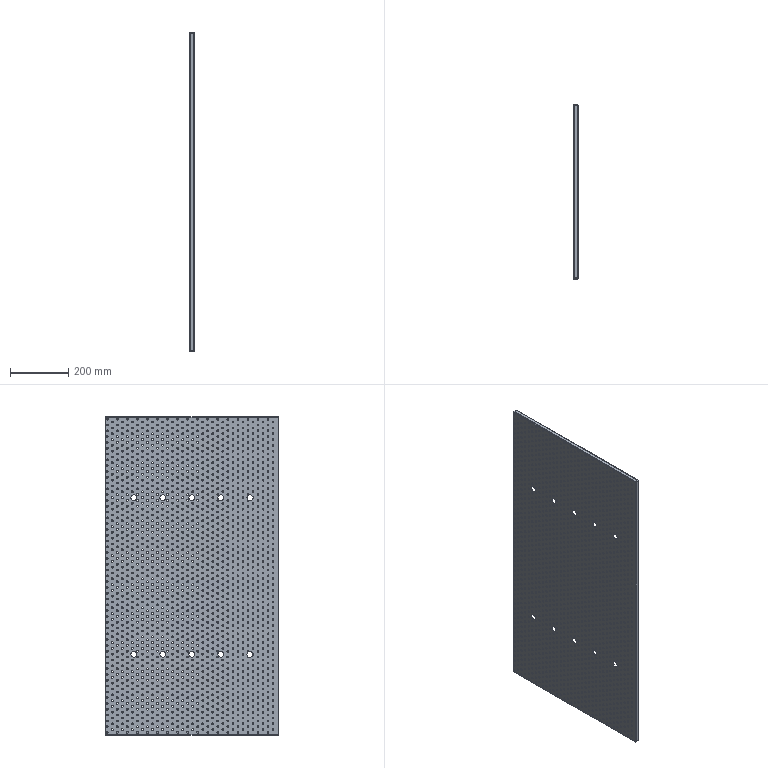Part | STEP file | HJDX-304 | 1 solid | 3784 faces | volume 1378157 mm3 | cylinder 3730 | plane 38 | spline 16 | commonest cylinder face diameters 6 x3690 20 x24 1 x8 5 x8